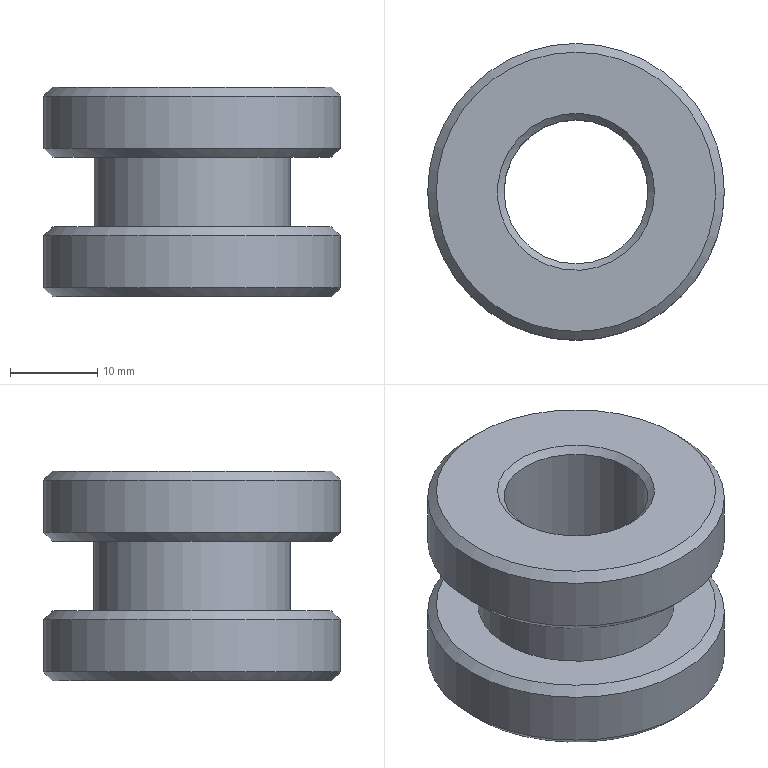Part | STEP file | YBQDJ-PD-16 | 1 solid | 14 faces | box 34 x 34 x 24 mm | volume 12336 mm3 | cone 6 | plane 4 | cylinder 4 | commonest cylinder face diameters 34 x2 16.5 x1 22.5 x1
STEP:
#1=CARTESIAN_POINT('',(0.,0.,0.));
#2=DIRECTION('',(0.,0.,1.));
#3=DIRECTION('',(1.,0.,0.));
#4=AXIS2_PLACEMENT_3D('',#1,#2,#3);
#5=CARTESIAN_POINT('',(-174.5,305.,279.5));
#6=VERTEX_POINT('',#5);
#7=CARTESIAN_POINT('',(-183.5,305.,279.5));
#8=DIRECTION('',(0.,0.,-1.));
#9=DIRECTION('',(1.,0.,0.));
#10=AXIS2_PLACEMENT_3D('',#7,#8,#9);
#11=CIRCLE('',#10,9.);
#12=CARTESIAN_POINT('',(-183.5,305.,279.5));
#13=DIRECTION('',(0.,0.,1.));
#14=DIRECTION('',(1.,0.,0.));
#15=AXIS2_PLACEMENT_3D('',#12,#13,#14);
#16=PLANE('',#15);
#17=CARTESIAN_POINT('',(9.,0.));
#18=CARTESIAN_POINT('',(9.,-15.588));
#19=CARTESIAN_POINT('',(-4.5,-7.794));
#20=CARTESIAN_POINT('',(-18.,0.));
#21=CARTESIAN_POINT('',(-4.5,7.794));
#22=CARTESIAN_POINT('',(9.,15.588));
#23=CARTESIAN_POINT('',(9.,0.));
#24=(BOUNDED_CURVE()B_SPLINE_CURVE(2,(#17,#18,#19,#20,#21,#22,#23),.UNSPECIFIED.,.T.,.F.)B_SPLINE_CURVE_WITH_KNOTS((1,2,2,2,2,1),(-2.094,0.,2.094,4.189,6.283,8.378),.UNSPECIFIED.)CURVE()GEOMETRIC_REPRESENTATION_ITEM()RATIONAL_B_SPLINE_CURVE((1.,0.5,1.,0.5,1.,0.5,1.))REPRESENTATION_ITEM(''));
#25=(GEOMETRIC_REPRESENTATION_CONTEXT(2)PARAMETRIC_REPRESENTATION_CONTEXT()REPRESENTATION_CONTEXT('',''));
#26=DEFINITIONAL_REPRESENTATION('',(#24),#25);
#27=PCURVE('',#16,#26);
#28=CARTESIAN_POINT('',(-183.5,305.,279.5));
#29=DIRECTION('',(0.,0.,1.));
#30=DIRECTION('',(1.,0.,0.));
#31=AXIS2_PLACEMENT_3D('',#28,#29,#30);
#32=CONICAL_SURFACE('',#31,9.,0.7854);
#33=CARTESIAN_POINT('',(6.283,0.));
#34=DIRECTION('',(-1.,0.));
#35=VECTOR('',#34,1.);
#36=LINE('',#33,#35);
#37=(GEOMETRIC_REPRESENTATION_CONTEXT(2)PARAMETRIC_REPRESENTATION_CONTEXT()REPRESENTATION_CONTEXT('',''));
#38=DEFINITIONAL_REPRESENTATION('',(#36),#37);
#39=PCURVE('',#32,#38);
#40=SURFACE_CURVE('',#11,(#27,#39),.PCURVE_S1.);
#41=EDGE_CURVE('',#6,#6,#40,.T.);
#42=ORIENTED_EDGE('',*,*,#41,.T.);
#43=EDGE_LOOP('',(#42));
#44=FACE_BOUND('',#43,.T.);
#45=CARTESIAN_POINT('',(-167.5,305.,279.5));
#46=VERTEX_POINT('',#45);
#47=CARTESIAN_POINT('',(-199.5,305.,279.5));
#48=VERTEX_POINT('',#47);
#49=CARTESIAN_POINT('',(-183.5,305.,279.5));
#50=DIRECTION('',(0.,0.,1.));
#51=DIRECTION('',(1.,0.,0.));
#52=AXIS2_PLACEMENT_3D('',#49,#50,#51);
#53=CIRCLE('',#52,16.);
#54=CARTESIAN_POINT('',(0.,0.));
#55=DIRECTION('',(1.,0.));
#56=AXIS2_PLACEMENT_2D('',#54,#55);
#57=CIRCLE('',#56,16.);
#58=(GEOMETRIC_REPRESENTATION_CONTEXT(2)PARAMETRIC_REPRESENTATION_CONTEXT()REPRESENTATION_CONTEXT('',''));
#59=DEFINITIONAL_REPRESENTATION('',(#57),#58);
#60=PCURVE('',#16,#59);
#61=CARTESIAN_POINT('',(-183.5,305.,279.5));
#62=DIRECTION('',(0.,0.,-1.));
#63=DIRECTION('',(-1.,0.,0.));
#64=AXIS2_PLACEMENT_3D('',#61,#62,#63);
#65=CONICAL_SURFACE('',#64,16.,0.7854);
#66=CARTESIAN_POINT('',(3.142,0.));
#67=DIRECTION('',(-1.,0.));
#68=VECTOR('',#67,1.);
#69=LINE('',#66,#68);
#70=(GEOMETRIC_REPRESENTATION_CONTEXT(2)PARAMETRIC_REPRESENTATION_CONTEXT()REPRESENTATION_CONTEXT('',''));
#71=DEFINITIONAL_REPRESENTATION('',(#69),#70);
#72=PCURVE('',#65,#71);
#73=SURFACE_CURVE('',#53,(#60,#72),.PCURVE_S1.);
#74=EDGE_CURVE('',#46,#48,#73,.T.);
#75=ORIENTED_EDGE('',*,*,#74,.T.);
#76=CARTESIAN_POINT('',(-183.5,305.,279.5));
#77=DIRECTION('',(0.,0.,1.));
#78=DIRECTION('',(1.,0.,0.));
#79=AXIS2_PLACEMENT_3D('',#76,#77,#78);
#80=CIRCLE('',#79,16.);
#81=CARTESIAN_POINT('',(0.,0.));
#82=DIRECTION('',(1.,0.));
#83=AXIS2_PLACEMENT_2D('',#81,#82);
#84=CIRCLE('',#83,16.);
#85=(GEOMETRIC_REPRESENTATION_CONTEXT(2)PARAMETRIC_REPRESENTATION_CONTEXT()REPRESENTATION_CONTEXT('',''));
#86=DEFINITIONAL_REPRESENTATION('',(#84),#85);
#87=PCURVE('',#16,#86);
#88=CARTESIAN_POINT('',(9.425,0.));
#89=DIRECTION('',(-1.,0.));
#90=VECTOR('',#89,1.);
#91=LINE('',#88,#90);
#92=(GEOMETRIC_REPRESENTATION_CONTEXT(2)PARAMETRIC_REPRESENTATION_CONTEXT()REPRESENTATION_CONTEXT('',''));
#93=DEFINITIONAL_REPRESENTATION('',(#91),#92);
#94=PCURVE('',#65,#93);
#95=SURFACE_CURVE('',#80,(#87,#94),.PCURVE_S1.);
#96=EDGE_CURVE('',#48,#46,#95,.T.);
#97=ORIENTED_EDGE('',*,*,#96,.T.);
#98=EDGE_LOOP('',(#75,#97));
#99=FACE_BOUND('',#98,.T.);
#100=ADVANCED_FACE('',(#44,#99),#16,.T.);
#101=CARTESIAN_POINT('',(-174.5,305.,255.5));
#102=VERTEX_POINT('',#101);
#103=CARTESIAN_POINT('',(-183.5,305.,255.5));
#104=DIRECTION('',(0.,0.,1.));
#105=DIRECTION('',(1.,0.,0.));
#106=AXIS2_PLACEMENT_3D('',#103,#104,#105);
#107=CIRCLE('',#106,9.);
#108=CARTESIAN_POINT('',(-183.5,305.,255.5));
#109=DIRECTION('',(0.,0.,1.));
#110=DIRECTION('',(1.,0.,0.));
#111=AXIS2_PLACEMENT_3D('',#108,#109,#110);
#112=PLANE('',#111);
#113=CARTESIAN_POINT('',(0.,0.));
#114=DIRECTION('',(1.,0.));
#115=AXIS2_PLACEMENT_2D('',#113,#114);
#116=CIRCLE('',#115,9.);
#117=(GEOMETRIC_REPRESENTATION_CONTEXT(2)PARAMETRIC_REPRESENTATION_CONTEXT()REPRESENTATION_CONTEXT('',''));
#118=DEFINITIONAL_REPRESENTATION('',(#116),#117);
#119=PCURVE('',#112,#118);
#120=CARTESIAN_POINT('',(-183.5,305.,255.5));
#121=DIRECTION('',(0.,0.,-1.));
#122=DIRECTION('',(-1.,0.,0.));
#123=AXIS2_PLACEMENT_3D('',#120,#121,#122);
#124=CONICAL_SURFACE('',#123,9.,0.7854);
#125=CARTESIAN_POINT('',(9.425,0.));
#126=DIRECTION('',(-1.,0.));
#127=VECTOR('',#126,1.);
#128=LINE('',#125,#127);
#129=(GEOMETRIC_REPRESENTATION_CONTEXT(2)PARAMETRIC_REPRESENTATION_CONTEXT()REPRESENTATION_CONTEXT('',''));
#130=DEFINITIONAL_REPRESENTATION('',(#128),#129);
#131=PCURVE('',#124,#130);
#132=SURFACE_CURVE('',#107,(#119,#131),.PCURVE_S1.);
#133=EDGE_CURVE('',#102,#102,#132,.T.);
#134=ORIENTED_EDGE('',*,*,#133,.T.);
#135=EDGE_LOOP('',(#134));
#136=FACE_BOUND('',#135,.T.);
#137=CARTESIAN_POINT('',(-167.5,305.,255.5));
#138=VERTEX_POINT('',#137);
#139=CARTESIAN_POINT('',(-183.5,305.,255.5));
#140=DIRECTION('',(0.,0.,-1.));
#141=DIRECTION('',(1.,0.,0.));
#142=AXIS2_PLACEMENT_3D('',#139,#140,#141);
#143=CIRCLE('',#142,16.);
#144=CARTESIAN_POINT('',(16.,0.));
#145=CARTESIAN_POINT('',(16.,-27.713));
#146=CARTESIAN_POINT('',(-8.,-13.856));
#147=CARTESIAN_POINT('',(-32.,0.));
#148=CARTESIAN_POINT('',(-8.,13.856));
#149=CARTESIAN_POINT('',(16.,27.713));
#150=CARTESIAN_POINT('',(16.,0.));
#151=(BOUNDED_CURVE()B_SPLINE_CURVE(2,(#144,#145,#146,#147,#148,#149,#150),.UNSPECIFIED.,.T.,.F.)B_SPLINE_CURVE_WITH_KNOTS((1,2,2,2,2,1),(-2.094,0.,2.094,4.189,6.283,8.378),.UNSPECIFIED.)CURVE()GEOMETRIC_REPRESENTATION_ITEM()RATIONAL_B_SPLINE_CURVE((1.,0.5,1.,0.5,1.,0.5,1.))REPRESENTATION_ITEM(''));
#152=(GEOMETRIC_REPRESENTATION_CONTEXT(2)PARAMETRIC_REPRESENTATION_CONTEXT()REPRESENTATION_CONTEXT('',''));
#153=DEFINITIONAL_REPRESENTATION('',(#151),#152);
#154=PCURVE('',#112,#153);
#155=CARTESIAN_POINT('',(-183.5,305.,256.5));
#156=DIRECTION('',(0.,0.,1.));
#157=DIRECTION('',(1.,0.,0.));
#158=AXIS2_PLACEMENT_3D('',#155,#156,#157);
#159=CONICAL_SURFACE('',#158,17.,0.7854);
#160=CARTESIAN_POINT('',(6.283,-1.));
#161=DIRECTION('',(-1.,0.));
#162=VECTOR('',#161,1.);
#163=LINE('',#160,#162);
#164=(GEOMETRIC_REPRESENTATION_CONTEXT(2)PARAMETRIC_REPRESENTATION_CONTEXT()REPRESENTATION_CONTEXT('',''));
#165=DEFINITIONAL_REPRESENTATION('',(#163),#164);
#166=PCURVE('',#159,#165);
#167=SURFACE_CURVE('',#143,(#154,#166),.PCURVE_S1.);
#168=EDGE_CURVE('',#138,#138,#167,.T.);
#169=ORIENTED_EDGE('',*,*,#168,.T.);
#170=EDGE_LOOP('',(#169));
#171=FACE_BOUND('',#170,.T.);
#172=ADVANCED_FACE('',(#136,#171),#112,.F.);
#173=CARTESIAN_POINT('',(-175.25,305.,256.25));
#174=VERTEX_POINT('',#173);
#175=CARTESIAN_POINT('',(-183.5,305.,256.25));
#176=DIRECTION('',(0.,0.,-1.));
#177=DIRECTION('',(1.,0.,0.));
#178=AXIS2_PLACEMENT_3D('',#175,#176,#177);
#179=CIRCLE('',#178,8.25);
#180=CARTESIAN_POINT('',(-183.5,305.,279.5));
#181=DIRECTION('',(0.,0.,-1.));
#182=DIRECTION('',(-1.,0.,0.));
#183=AXIS2_PLACEMENT_3D('',#180,#181,#182);
#184=CYLINDRICAL_SURFACE('',#183,8.25);
#185=CARTESIAN_POINT('',(3.142,23.25));
#186=DIRECTION('',(1.,0.));
#187=VECTOR('',#186,1.);
#188=LINE('',#185,#187);
#189=(GEOMETRIC_REPRESENTATION_CONTEXT(2)PARAMETRIC_REPRESENTATION_CONTEXT()REPRESENTATION_CONTEXT('',''));
#190=DEFINITIONAL_REPRESENTATION('',(#188),#189);
#191=PCURVE('',#184,#190);
#192=CARTESIAN_POINT('',(3.142,-0.75));
#193=DIRECTION('',(1.,0.));
#194=VECTOR('',#193,1.);
#195=LINE('',#192,#194);
#196=(GEOMETRIC_REPRESENTATION_CONTEXT(2)PARAMETRIC_REPRESENTATION_CONTEXT()REPRESENTATION_CONTEXT('',''));
#197=DEFINITIONAL_REPRESENTATION('',(#195),#196);
#198=PCURVE('',#124,#197);
#199=SURFACE_CURVE('',#179,(#191,#198),.PCURVE_S1.);
#200=EDGE_CURVE('',#174,#174,#199,.T.);
#201=ORIENTED_EDGE('',*,*,#200,.F.);
#202=CARTESIAN_POINT('',(-175.25,305.,278.75));
#203=VERTEX_POINT('',#202);
#204=CARTESIAN_POINT('',(-175.25,305.,278.75));
#205=CARTESIAN_POINT('',(-175.25,305.,256.25));
#206=B_SPLINE_CURVE_WITH_KNOTS('',1,(#204,#205),.UNSPECIFIED.,.F.,.F.,(2,2),(0.75,23.25),.PIECEWISE_BEZIER_KNOTS.);
#207=CARTESIAN_POINT('',(3.142,0.));
#208=DIRECTION('',(0.,1.));
#209=VECTOR('',#208,1.);
#210=LINE('',#207,#209);
#211=(GEOMETRIC_REPRESENTATION_CONTEXT(2)PARAMETRIC_REPRESENTATION_CONTEXT()REPRESENTATION_CONTEXT('',''));
#212=DEFINITIONAL_REPRESENTATION('',(#210),#211);
#213=PCURVE('',#184,#212);
#214=CARTESIAN_POINT('',(9.425,0.));
#215=DIRECTION('',(0.,1.));
#216=VECTOR('',#215,1.);
#217=LINE('',#214,#216);
#218=(GEOMETRIC_REPRESENTATION_CONTEXT(2)PARAMETRIC_REPRESENTATION_CONTEXT()REPRESENTATION_CONTEXT('',''));
#219=DEFINITIONAL_REPRESENTATION('',(#217),#218);
#220=PCURVE('',#184,#219);
#221=SEAM_CURVE('',#206,(#213,#220),.PCURVE_S1.);
#222=EDGE_CURVE('',#203,#174,#221,.T.);
#223=ORIENTED_EDGE('',*,*,#222,.F.);
#224=CARTESIAN_POINT('',(-183.5,305.,278.75));
#225=DIRECTION('',(0.,0.,1.));
#226=DIRECTION('',(1.,0.,0.));
#227=AXIS2_PLACEMENT_3D('',#224,#225,#226);
#228=CIRCLE('',#227,8.25);
#229=CARTESIAN_POINT('',(9.425,0.75));
#230=DIRECTION('',(-1.,0.));
#231=VECTOR('',#230,1.);
#232=LINE('',#229,#231);
#233=(GEOMETRIC_REPRESENTATION_CONTEXT(2)PARAMETRIC_REPRESENTATION_CONTEXT()REPRESENTATION_CONTEXT('',''));
#234=DEFINITIONAL_REPRESENTATION('',(#232),#233);
#235=PCURVE('',#184,#234);
#236=CARTESIAN_POINT('',(0.,-0.75));
#237=DIRECTION('',(1.,0.));
#238=VECTOR('',#237,1.);
#239=LINE('',#236,#238);
#240=(GEOMETRIC_REPRESENTATION_CONTEXT(2)PARAMETRIC_REPRESENTATION_CONTEXT()REPRESENTATION_CONTEXT('',''));
#241=DEFINITIONAL_REPRESENTATION('',(#239),#240);
#242=PCURVE('',#32,#241);
#243=SURFACE_CURVE('',#228,(#235,#242),.PCURVE_S1.);
#244=EDGE_CURVE('',#203,#203,#243,.T.);
#245=ORIENTED_EDGE('',*,*,#244,.F.);
#246=ORIENTED_EDGE('',*,*,#222,.T.);
#247=EDGE_LOOP('',(#201,#223,#245,#246));
#248=FACE_BOUND('',#247,.F.);
#249=ADVANCED_FACE('',(#248),#184,.F.);
#250=CARTESIAN_POINT('',(-166.5,305.,272.5));
#251=VERTEX_POINT('',#250);
#252=CARTESIAN_POINT('',(-200.5,305.,272.5));
#253=VERTEX_POINT('',#252);
#254=CARTESIAN_POINT('',(-183.5,305.,272.5));
#255=DIRECTION('',(0.,0.,1.));
#256=DIRECTION('',(1.,0.,0.));
#257=AXIS2_PLACEMENT_3D('',#254,#255,#256);
#258=CIRCLE('',#257,17.);
#259=CARTESIAN_POINT('',(-183.5,305.,279.5));
#260=DIRECTION('',(0.,0.,-1.));
#261=DIRECTION('',(-1.,0.,0.));
#262=AXIS2_PLACEMENT_3D('',#259,#260,#261);
#263=CYLINDRICAL_SURFACE('',#262,17.);
#264=CARTESIAN_POINT('',(3.142,7.));
#265=DIRECTION('',(-1.,0.));
#266=VECTOR('',#265,1.);
#267=LINE('',#264,#266);
#268=(GEOMETRIC_REPRESENTATION_CONTEXT(2)PARAMETRIC_REPRESENTATION_CONTEXT()REPRESENTATION_CONTEXT('',''));
#269=DEFINITIONAL_REPRESENTATION('',(#267),#268);
#270=PCURVE('',#263,#269);
#271=CARTESIAN_POINT('',(-183.5,305.,272.5));
#272=DIRECTION('',(0.,0.,1.));
#273=DIRECTION('',(1.,0.,0.));
#274=AXIS2_PLACEMENT_3D('',#271,#272,#273);
#275=CONICAL_SURFACE('',#274,17.,0.7854);
#276=CARTESIAN_POINT('',(0.,0.));
#277=DIRECTION('',(1.,0.));
#278=VECTOR('',#277,1.);
#279=LINE('',#276,#278);
#280=(GEOMETRIC_REPRESENTATION_CONTEXT(2)PARAMETRIC_REPRESENTATION_CONTEXT()REPRESENTATION_CONTEXT('',''));
#281=DEFINITIONAL_REPRESENTATION('',(#279),#280);
#282=PCURVE('',#275,#281);
#283=SURFACE_CURVE('',#258,(#270,#282),.PCURVE_S1.);
#284=EDGE_CURVE('',#251,#253,#283,.T.);
#285=ORIENTED_EDGE('',*,*,#284,.T.);
#286=CARTESIAN_POINT('',(-200.5,305.,278.5));
#287=VERTEX_POINT('',#286);
#288=CARTESIAN_POINT('',(-200.5,305.,278.5));
#289=CARTESIAN_POINT('',(-200.5,305.,272.5));
#290=B_SPLINE_CURVE_WITH_KNOTS('',1,(#288,#289),.UNSPECIFIED.,.F.,.F.,(2,2),(1.,7.),.PIECEWISE_BEZIER_KNOTS.);
#291=CARTESIAN_POINT('',(0.,0.));
#292=DIRECTION('',(0.,1.));
#293=VECTOR('',#292,1.);
#294=LINE('',#291,#293);
#295=(GEOMETRIC_REPRESENTATION_CONTEXT(2)PARAMETRIC_REPRESENTATION_CONTEXT()REPRESENTATION_CONTEXT('',''));
#296=DEFINITIONAL_REPRESENTATION('',(#294),#295);
#297=PCURVE('',#263,#296);
#298=CARTESIAN_POINT('',(6.283,0.));
#299=DIRECTION('',(0.,1.));
#300=VECTOR('',#299,1.);
#301=LINE('',#298,#300);
#302=(GEOMETRIC_REPRESENTATION_CONTEXT(2)PARAMETRIC_REPRESENTATION_CONTEXT()REPRESENTATION_CONTEXT('',''));
#303=DEFINITIONAL_REPRESENTATION('',(#301),#302);
#304=PCURVE('',#263,#303);
#305=SEAM_CURVE('',#290,(#297,#304),.PCURVE_S1.);
#306=EDGE_CURVE('',#287,#253,#305,.T.);
#307=ORIENTED_EDGE('',*,*,#306,.F.);
#308=CARTESIAN_POINT('',(-183.5,305.,278.5));
#309=DIRECTION('',(0.,0.,-1.));
#310=DIRECTION('',(-1.,0.,0.));
#311=AXIS2_PLACEMENT_3D('',#308,#309,#310);
#312=CIRCLE('',#311,17.);
#313=CARTESIAN_POINT('',(0.,1.));
#314=DIRECTION('',(1.,0.));
#315=VECTOR('',#314,1.);
#316=LINE('',#313,#315);
#317=(GEOMETRIC_REPRESENTATION_CONTEXT(2)PARAMETRIC_REPRESENTATION_CONTEXT()REPRESENTATION_CONTEXT('',''));
#318=DEFINITIONAL_REPRESENTATION('',(#316),#317);
#319=PCURVE('',#263,#318);
#320=CARTESIAN_POINT('',(0.,1.));
#321=DIRECTION('',(1.,0.));
#322=VECTOR('',#321,1.);
#323=LINE('',#320,#322);
#324=(GEOMETRIC_REPRESENTATION_CONTEXT(2)PARAMETRIC_REPRESENTATION_CONTEXT()REPRESENTATION_CONTEXT('',''));
#325=DEFINITIONAL_REPRESENTATION('',(#323),#324);
#326=PCURVE('',#65,#325);
#327=SURFACE_CURVE('',#312,(#319,#326),.PCURVE_S1.);
#328=EDGE_CURVE('',#287,#287,#327,.T.);
#329=ORIENTED_EDGE('',*,*,#328,.T.);
#330=ORIENTED_EDGE('',*,*,#306,.T.);
#331=CARTESIAN_POINT('',(-183.5,305.,272.5));
#332=DIRECTION('',(0.,0.,1.));
#333=DIRECTION('',(1.,0.,0.));
#334=AXIS2_PLACEMENT_3D('',#331,#332,#333);
#335=CIRCLE('',#334,17.);
#336=CARTESIAN_POINT('',(9.425,7.));
#337=DIRECTION('',(-1.,0.));
#338=VECTOR('',#337,1.);
#339=LINE('',#336,#338);
#340=(GEOMETRIC_REPRESENTATION_CONTEXT(2)PARAMETRIC_REPRESENTATION_CONTEXT()REPRESENTATION_CONTEXT('',''));
#341=DEFINITIONAL_REPRESENTATION('',(#339),#340);
#342=PCURVE('',#263,#341);
#343=CARTESIAN_POINT('',(0.,0.));
#344=DIRECTION('',(1.,0.));
#345=VECTOR('',#344,1.);
#346=LINE('',#343,#345);
#347=(GEOMETRIC_REPRESENTATION_CONTEXT(2)PARAMETRIC_REPRESENTATION_CONTEXT()REPRESENTATION_CONTEXT('',''));
#348=DEFINITIONAL_REPRESENTATION('',(#346),#347);
#349=PCURVE('',#275,#348);
#350=SURFACE_CURVE('',#335,(#342,#349),.PCURVE_S1.);
#351=EDGE_CURVE('',#253,#251,#350,.T.);
#352=ORIENTED_EDGE('',*,*,#351,.T.);
#353=EDGE_LOOP('',(#285,#307,#329,#330,#352));
#354=FACE_BOUND('',#353,.T.);
#355=ADVANCED_FACE('',(#354),#263,.T.);
#356=CARTESIAN_POINT('',(-167.5,305.,271.5));
#357=VERTEX_POINT('',#356);
#358=CARTESIAN_POINT('',(-183.5,305.,271.5));
#359=DIRECTION('',(0.,0.,-1.));
#360=DIRECTION('',(1.,0.,0.));
#361=AXIS2_PLACEMENT_3D('',#358,#359,#360);
#362=CIRCLE('',#361,16.);
#363=CARTESIAN_POINT('',(-183.5,305.,271.5));
#364=DIRECTION('',(0.,0.,1.));
#365=DIRECTION('',(1.,0.,0.));
#366=AXIS2_PLACEMENT_3D('',#363,#364,#365);
#367=PLANE('',#366);
#368=CARTESIAN_POINT('',(16.,0.));
#369=CARTESIAN_POINT('',(16.,-27.713));
#370=CARTESIAN_POINT('',(-8.,-13.856));
#371=CARTESIAN_POINT('',(-32.,0.));
#372=CARTESIAN_POINT('',(-8.,13.856));
#373=CARTESIAN_POINT('',(16.,27.713));
#374=CARTESIAN_POINT('',(16.,0.));
#375=(BOUNDED_CURVE()B_SPLINE_CURVE(2,(#368,#369,#370,#371,#372,#373,#374),.UNSPECIFIED.,.T.,.F.)B_SPLINE_CURVE_WITH_KNOTS((1,2,2,2,2,1),(-2.094,0.,2.094,4.189,6.283,8.378),.UNSPECIFIED.)CURVE()GEOMETRIC_REPRESENTATION_ITEM()RATIONAL_B_SPLINE_CURVE((1.,0.5,1.,0.5,1.,0.5,1.))REPRESENTATION_ITEM(''));
#376=(GEOMETRIC_REPRESENTATION_CONTEXT(2)PARAMETRIC_REPRESENTATION_CONTEXT()REPRESENTATION_CONTEXT('',''));
#377=DEFINITIONAL_REPRESENTATION('',(#375),#376);
#378=PCURVE('',#367,#377);
#379=CARTESIAN_POINT('',(6.283,-1.));
#380=DIRECTION('',(-1.,0.));
#381=VECTOR('',#380,1.);
#382=LINE('',#379,#381);
#383=(GEOMETRIC_REPRESENTATION_CONTEXT(2)PARAMETRIC_REPRESENTATION_CONTEXT()REPRESENTATION_CONTEXT('',''));
#384=DEFINITIONAL_REPRESENTATION('',(#382),#383);
#385=PCURVE('',#275,#384);
#386=SURFACE_CURVE('',#362,(#378,#385),.PCURVE_S1.);
#387=EDGE_CURVE('',#357,#357,#386,.T.);
#388=ORIENTED_EDGE('',*,*,#387,.T.);
#389=EDGE_LOOP('',(#388));
#390=FACE_BOUND('',#389,.T.);
#391=CARTESIAN_POINT('',(-172.25,305.,271.5));
#392=VERTEX_POINT('',#391);
#393=CARTESIAN_POINT('',(-183.5,305.,271.5));
#394=DIRECTION('',(0.,0.,1.));
#395=DIRECTION('',(1.,0.,0.));
#396=AXIS2_PLACEMENT_3D('',#393,#394,#395);
#397=CIRCLE('',#396,11.25);
#398=CARTESIAN_POINT('',(0.,0.));
#399=DIRECTION('',(1.,0.));
#400=AXIS2_PLACEMENT_2D('',#398,#399);
#401=CIRCLE('',#400,11.25);
#402=(GEOMETRIC_REPRESENTATION_CONTEXT(2)PARAMETRIC_REPRESENTATION_CONTEXT()REPRESENTATION_CONTEXT('',''));
#403=DEFINITIONAL_REPRESENTATION('',(#401),#402);
#404=PCURVE('',#367,#403);
#405=CARTESIAN_POINT('',(-183.5,305.,271.5));
#406=DIRECTION('',(0.,0.,-1.));
#407=DIRECTION('',(-1.,0.,0.));
#408=AXIS2_PLACEMENT_3D('',#405,#406,#407);
#409=CYLINDRICAL_SURFACE('',#408,11.25);
#410=CARTESIAN_POINT('',(9.425,0.));
#411=DIRECTION('',(-1.,0.));
#412=VECTOR('',#411,1.);
#413=LINE('',#410,#412);
#414=(GEOMETRIC_REPRESENTATION_CONTEXT(2)PARAMETRIC_REPRESENTATION_CONTEXT()REPRESENTATION_CONTEXT('',''));
#415=DEFINITIONAL_REPRESENTATION('',(#413),#414);
#416=PCURVE('',#409,#415);
#417=SURFACE_CURVE('',#397,(#404,#416),.PCURVE_S1.);
#418=EDGE_CURVE('',#392,#392,#417,.T.);
#419=ORIENTED_EDGE('',*,*,#418,.T.);
#420=EDGE_LOOP('',(#419));
#421=FACE_BOUND('',#420,.T.);
#422=ADVANCED_FACE('',(#390,#421),#367,.F.);
#423=CARTESIAN_POINT('',(-166.5,305.,256.5));
#424=VERTEX_POINT('',#423);
#425=CARTESIAN_POINT('',(-200.5,305.,256.5));
#426=VERTEX_POINT('',#425);
#427=CARTESIAN_POINT('',(-183.5,305.,256.5));
#428=DIRECTION('',(0.,0.,1.));
#429=DIRECTION('',(1.,0.,0.));
#430=AXIS2_PLACEMENT_3D('',#427,#428,#429);
#431=CIRCLE('',#430,17.);
#432=CARTESIAN_POINT('',(-183.5,305.,263.5));
#433=DIRECTION('',(0.,0.,-1.));
#434=DIRECTION('',(-1.,0.,0.));
#435=AXIS2_PLACEMENT_3D('',#432,#433,#434);
#436=CYLINDRICAL_SURFACE('',#435,17.);
#437=CARTESIAN_POINT('',(3.142,7.));
#438=DIRECTION('',(-1.,0.));
#439=VECTOR('',#438,1.);
#440=LINE('',#437,#439);
#441=(GEOMETRIC_REPRESENTATION_CONTEXT(2)PARAMETRIC_REPRESENTATION_CONTEXT()REPRESENTATION_CONTEXT('',''));
#442=DEFINITIONAL_REPRESENTATION('',(#440),#441);
#443=PCURVE('',#436,#442);
#444=CARTESIAN_POINT('',(0.,0.));
#445=DIRECTION('',(1.,0.));
#446=VECTOR('',#445,1.);
#447=LINE('',#444,#446);
#448=(GEOMETRIC_REPRESENTATION_CONTEXT(2)PARAMETRIC_REPRESENTATION_CONTEXT()REPRESENTATION_CONTEXT('',''));
#449=DEFINITIONAL_REPRESENTATION('',(#447),#448);
#450=PCURVE('',#159,#449);
#451=SURFACE_CURVE('',#431,(#443,#450),.PCURVE_S1.);
#452=EDGE_CURVE('',#424,#426,#451,.T.);
#453=ORIENTED_EDGE('',*,*,#452,.T.);
#454=CARTESIAN_POINT('',(-200.5,305.,262.5));
#455=VERTEX_POINT('',#454);
#456=CARTESIAN_POINT('',(-200.5,305.,262.5));
#457=CARTESIAN_POINT('',(-200.5,305.,256.5));
#458=B_SPLINE_CURVE_WITH_KNOTS('',1,(#456,#457),.UNSPECIFIED.,.F.,.F.,(2,2),(1.,7.),.PIECEWISE_BEZIER_KNOTS.);
#459=CARTESIAN_POINT('',(0.,0.));
#460=DIRECTION('',(0.,1.));
#461=VECTOR('',#460,1.);
#462=LINE('',#459,#461);
#463=(GEOMETRIC_REPRESENTATION_CONTEXT(2)PARAMETRIC_REPRESENTATION_CONTEXT()REPRESENTATION_CONTEXT('',''));
#464=DEFINITIONAL_REPRESENTATION('',(#462),#463);
#465=PCURVE('',#436,#464);
#466=CARTESIAN_POINT('',(6.283,0.));
#467=DIRECTION('',(0.,1.));
#468=VECTOR('',#467,1.);
#469=LINE('',#466,#468);
#470=(GEOMETRIC_REPRESENTATION_CONTEXT(2)PARAMETRIC_REPRESENTATION_CONTEXT()REPRESENTATION_CONTEXT('',''));
#471=DEFINITIONAL_REPRESENTATION('',(#469),#470);
#472=PCURVE('',#436,#471);
#473=SEAM_CURVE('',#458,(#465,#472),.PCURVE_S1.);
#474=EDGE_CURVE('',#455,#426,#473,.T.);
#475=ORIENTED_EDGE('',*,*,#474,.F.);
#476=CARTESIAN_POINT('',(-183.5,305.,262.5));
#477=DIRECTION('',(0.,0.,-1.));
#478=DIRECTION('',(-1.,0.,0.));
#479=AXIS2_PLACEMENT_3D('',#476,#477,#478);
#480=CIRCLE('',#479,17.);
#481=CARTESIAN_POINT('',(0.,1.));
#482=DIRECTION('',(1.,0.));
#483=VECTOR('',#482,1.);
#484=LINE('',#481,#483);
#485=(GEOMETRIC_REPRESENTATION_CONTEXT(2)PARAMETRIC_REPRESENTATION_CONTEXT()REPRESENTATION_CONTEXT('',''));
#486=DEFINITIONAL_REPRESENTATION('',(#484),#485);
#487=PCURVE('',#436,#486);
#488=CARTESIAN_POINT('',(-183.5,305.,263.5));
#489=DIRECTION('',(0.,0.,-1.));
#490=DIRECTION('',(-1.,0.,0.));
#491=AXIS2_PLACEMENT_3D('',#488,#489,#490);
#492=CONICAL_SURFACE('',#491,16.,0.7854);
#493=CARTESIAN_POINT('',(0.,1.));
#494=DIRECTION('',(1.,0.));
#495=VECTOR('',#494,1.);
#496=LINE('',#493,#495);
#497=(GEOMETRIC_REPRESENTATION_CONTEXT(2)PARAMETRIC_REPRESENTATION_CONTEXT()REPRESENTATION_CONTEXT('',''));
#498=DEFINITIONAL_REPRESENTATION('',(#496),#497);
#499=PCURVE('',#492,#498);
#500=SURFACE_CURVE('',#480,(#487,#499),.PCURVE_S1.);
#501=EDGE_CURVE('',#455,#455,#500,.T.);
#502=ORIENTED_EDGE('',*,*,#501,.T.);
#503=ORIENTED_EDGE('',*,*,#474,.T.);
#504=CARTESIAN_POINT('',(-183.5,305.,256.5));
#505=DIRECTION('',(0.,0.,1.));
#506=DIRECTION('',(1.,0.,0.));
#507=AXIS2_PLACEMENT_3D('',#504,#505,#506);
#508=CIRCLE('',#507,17.);
#509=CARTESIAN_POINT('',(9.425,7.));
#510=DIRECTION('',(-1.,0.));
#511=VECTOR('',#510,1.);
#512=LINE('',#509,#511);
#513=(GEOMETRIC_REPRESENTATION_CONTEXT(2)PARAMETRIC_REPRESENTATION_CONTEXT()REPRESENTATION_CONTEXT('',''));
#514=DEFINITIONAL_REPRESENTATION('',(#512),#513);
#515=PCURVE('',#436,#514);
#516=CARTESIAN_POINT('',(0.,0.));
#517=DIRECTION('',(1.,0.));
#518=VECTOR('',#517,1.);
#519=LINE('',#516,#518);
#520=(GEOMETRIC_REPRESENTATION_CONTEXT(2)PARAMETRIC_REPRESENTATION_CONTEXT()REPRESENTATION_CONTEXT('',''));
#521=DEFINITIONAL_REPRESENTATION('',(#519),#520);
#522=PCURVE('',#159,#521);
#523=SURFACE_CURVE('',#508,(#515,#522),.PCURVE_S1.);
#524=EDGE_CURVE('',#426,#424,#523,.T.);
#525=ORIENTED_EDGE('',*,*,#524,.T.);
#526=EDGE_LOOP('',(#453,#475,#502,#503,#525));
#527=FACE_BOUND('',#526,.T.);
#528=ADVANCED_FACE('',(#527),#436,.T.);
#529=CARTESIAN_POINT('',(-167.5,305.,263.5));
#530=VERTEX_POINT('',#529);
#531=CARTESIAN_POINT('',(-199.5,305.,263.5));
#532=VERTEX_POINT('',#531);
#533=CARTESIAN_POINT('',(-183.5,305.,263.5));
#534=DIRECTION('',(0.,0.,1.));
#535=DIRECTION('',(1.,0.,0.));
#536=AXIS2_PLACEMENT_3D('',#533,#534,#535);
#537=CIRCLE('',#536,16.);
#538=CARTESIAN_POINT('',(-183.5,305.,263.5));
#539=DIRECTION('',(0.,0.,1.));
#540=DIRECTION('',(1.,0.,0.));
#541=AXIS2_PLACEMENT_3D('',#538,#539,#540);
#542=PLANE('',#541);
#543=CARTESIAN_POINT('',(0.,0.));
#544=DIRECTION('',(1.,0.));
#545=AXIS2_PLACEMENT_2D('',#543,#544);
#546=CIRCLE('',#545,16.);
#547=(GEOMETRIC_REPRESENTATION_CONTEXT(2)PARAMETRIC_REPRESENTATION_CONTEXT()REPRESENTATION_CONTEXT('',''));
#548=DEFINITIONAL_REPRESENTATION('',(#546),#547);
#549=PCURVE('',#542,#548);
#550=CARTESIAN_POINT('',(3.142,0.));
#551=DIRECTION('',(-1.,0.));
#552=VECTOR('',#551,1.);
#553=LINE('',#550,#552);
#554=(GEOMETRIC_REPRESENTATION_CONTEXT(2)PARAMETRIC_REPRESENTATION_CONTEXT()REPRESENTATION_CONTEXT('',''));
#555=DEFINITIONAL_REPRESENTATION('',(#553),#554);
#556=PCURVE('',#492,#555);
#557=SURFACE_CURVE('',#537,(#549,#556),.PCURVE_S1.);
#558=EDGE_CURVE('',#530,#532,#557,.T.);
#559=ORIENTED_EDGE('',*,*,#558,.T.);
#560=CARTESIAN_POINT('',(-183.5,305.,263.5));
#561=DIRECTION('',(0.,0.,1.));
#562=DIRECTION('',(1.,0.,0.));
#563=AXIS2_PLACEMENT_3D('',#560,#561,#562);
#564=CIRCLE('',#563,16.);
#565=CARTESIAN_POINT('',(0.,0.));
#566=DIRECTION('',(1.,0.));
#567=AXIS2_PLACEMENT_2D('',#565,#566);
#568=CIRCLE('',#567,16.);
#569=(GEOMETRIC_REPRESENTATION_CONTEXT(2)PARAMETRIC_REPRESENTATION_CONTEXT()REPRESENTATION_CONTEXT('',''));
#570=DEFINITIONAL_REPRESENTATION('',(#568),#569);
#571=PCURVE('',#542,#570);
#572=CARTESIAN_POINT('',(9.425,0.));
#573=DIRECTION('',(-1.,0.));
#574=VECTOR('',#573,1.);
#575=LINE('',#572,#574);
#576=(GEOMETRIC_REPRESENTATION_CONTEXT(2)PARAMETRIC_REPRESENTATION_CONTEXT()REPRESENTATION_CONTEXT('',''));
#577=DEFINITIONAL_REPRESENTATION('',(#575),#576);
#578=PCURVE('',#492,#577);
#579=SURFACE_CURVE('',#564,(#571,#578),.PCURVE_S1.);
#580=EDGE_CURVE('',#532,#530,#579,.T.);
#581=ORIENTED_EDGE('',*,*,#580,.T.);
#582=EDGE_LOOP('',(#559,#581));
#583=FACE_BOUND('',#582,.T.);
#584=CARTESIAN_POINT('',(-172.25,305.,263.5));
#585=VERTEX_POINT('',#584);
#586=CARTESIAN_POINT('',(-183.5,305.,263.5));
#587=DIRECTION('',(0.,0.,1.));
#588=DIRECTION('',(1.,0.,0.));
#589=AXIS2_PLACEMENT_3D('',#586,#587,#588);
#590=CIRCLE('',#589,11.25);
#591=CARTESIAN_POINT('',(0.,0.));
#592=DIRECTION('',(1.,0.));
#593=AXIS2_PLACEMENT_2D('',#591,#592);
#594=CIRCLE('',#593,11.25);
#595=(GEOMETRIC_REPRESENTATION_CONTEXT(2)PARAMETRIC_REPRESENTATION_CONTEXT()REPRESENTATION_CONTEXT('',''));
#596=DEFINITIONAL_REPRESENTATION('',(#594),#595);
#597=PCURVE('',#542,#596);
#598=CARTESIAN_POINT('',(9.425,8.));
#599=DIRECTION('',(-1.,0.));
#600=VECTOR('',#599,1.);
#601=LINE('',#598,#600);
#602=(GEOMETRIC_REPRESENTATION_CONTEXT(2)PARAMETRIC_REPRESENTATION_CONTEXT()REPRESENTATION_CONTEXT('',''));
#603=DEFINITIONAL_REPRESENTATION('',(#601),#602);
#604=PCURVE('',#409,#603);
#605=SURFACE_CURVE('',#590,(#597,#604),.PCURVE_S1.);
#606=EDGE_CURVE('',#585,#585,#605,.T.);
#607=ORIENTED_EDGE('',*,*,#606,.F.);
#608=EDGE_LOOP('',(#607));
#609=FACE_BOUND('',#608,.T.);
#610=ADVANCED_FACE('',(#583,#609),#542,.T.);
#611=ORIENTED_EDGE('',*,*,#418,.F.);
#612=CARTESIAN_POINT('',(-172.25,305.,271.5));
#613=CARTESIAN_POINT('',(-172.25,305.,263.5));
#614=B_SPLINE_CURVE_WITH_KNOTS('',1,(#612,#613),.UNSPECIFIED.,.F.,.F.,(2,2),(0.,8.),.PIECEWISE_BEZIER_KNOTS.);
#615=CARTESIAN_POINT('',(9.425,0.));
#616=DIRECTION('',(0.,1.));
#617=VECTOR('',#616,1.);
#618=LINE('',#615,#617);
#619=(GEOMETRIC_REPRESENTATION_CONTEXT(2)PARAMETRIC_REPRESENTATION_CONTEXT()REPRESENTATION_CONTEXT('',''));
#620=DEFINITIONAL_REPRESENTATION('',(#618),#619);
#621=PCURVE('',#409,#620);
#622=CARTESIAN_POINT('',(3.142,0.));
#623=DIRECTION('',(0.,1.));
#624=VECTOR('',#623,1.);
#625=LINE('',#622,#624);
#626=(GEOMETRIC_REPRESENTATION_CONTEXT(2)PARAMETRIC_REPRESENTATION_CONTEXT()REPRESENTATION_CONTEXT('',''));
#627=DEFINITIONAL_REPRESENTATION('',(#625),#626);
#628=PCURVE('',#409,#627);
#629=SEAM_CURVE('',#614,(#621,#628),.PCURVE_S1.);
#630=EDGE_CURVE('',#392,#585,#629,.T.);
#631=ORIENTED_EDGE('',*,*,#630,.T.);
#632=ORIENTED_EDGE('',*,*,#606,.T.);
#633=ORIENTED_EDGE('',*,*,#630,.F.);
#634=EDGE_LOOP('',(#611,#631,#632,#633));
#635=FACE_BOUND('',#634,.T.);
#636=ADVANCED_FACE('',(#635),#409,.T.);
#637=ORIENTED_EDGE('',*,*,#168,.F.);
#638=CARTESIAN_POINT('',(-167.5,305.,255.5));
#639=CARTESIAN_POINT('',(-166.5,305.,256.5));
#640=B_SPLINE_CURVE_WITH_KNOTS('',1,(#638,#639),.UNSPECIFIED.,.F.,.F.,(2,2),(-1.414,0.),.PIECEWISE_BEZIER_KNOTS.);
#641=CARTESIAN_POINT('',(6.283,0.));
#642=DIRECTION('',(0.,1.));
#643=VECTOR('',#642,1.);
#644=LINE('',#641,#643);
#645=(GEOMETRIC_REPRESENTATION_CONTEXT(2)PARAMETRIC_REPRESENTATION_CONTEXT()REPRESENTATION_CONTEXT('',''));
#646=DEFINITIONAL_REPRESENTATION('',(#644),#645);
#647=PCURVE('',#159,#646);
#648=CARTESIAN_POINT('',(0.,0.));
#649=DIRECTION('',(0.,1.));
#650=VECTOR('',#649,1.);
#651=LINE('',#648,#650);
#652=(GEOMETRIC_REPRESENTATION_CONTEXT(2)PARAMETRIC_REPRESENTATION_CONTEXT()REPRESENTATION_CONTEXT('',''));
#653=DEFINITIONAL_REPRESENTATION('',(#651),#652);
#654=PCURVE('',#159,#653);
#655=SEAM_CURVE('',#640,(#647,#654),.PCURVE_S1.);
#656=EDGE_CURVE('',#138,#424,#655,.T.);
#657=ORIENTED_EDGE('',*,*,#656,.T.);
#658=ORIENTED_EDGE('',*,*,#524,.F.);
#659=ORIENTED_EDGE('',*,*,#452,.F.);
#660=ORIENTED_EDGE('',*,*,#656,.F.);
#661=EDGE_LOOP('',(#637,#657,#658,#659,#660));
#662=FACE_BOUND('',#661,.T.);
#663=ADVANCED_FACE('',(#662),#159,.T.);
#664=ORIENTED_EDGE('',*,*,#501,.F.);
#665=CARTESIAN_POINT('',(-199.5,305.,263.5));
#666=CARTESIAN_POINT('',(-200.5,305.,262.5));
#667=B_SPLINE_CURVE_WITH_KNOTS('',1,(#665,#666),.UNSPECIFIED.,.F.,.F.,(2,2),(0.,1.414),.PIECEWISE_BEZIER_KNOTS.);
#668=CARTESIAN_POINT('',(0.,0.));
#669=DIRECTION('',(0.,1.));
#670=VECTOR('',#669,1.);
#671=LINE('',#668,#670);
#672=(GEOMETRIC_REPRESENTATION_CONTEXT(2)PARAMETRIC_REPRESENTATION_CONTEXT()REPRESENTATION_CONTEXT('',''));
#673=DEFINITIONAL_REPRESENTATION('',(#671),#672);
#674=PCURVE('',#492,#673);
#675=CARTESIAN_POINT('',(6.283,0.));
#676=DIRECTION('',(0.,1.));
#677=VECTOR('',#676,1.);
#678=LINE('',#675,#677);
#679=(GEOMETRIC_REPRESENTATION_CONTEXT(2)PARAMETRIC_REPRESENTATION_CONTEXT()REPRESENTATION_CONTEXT('',''));
#680=DEFINITIONAL_REPRESENTATION('',(#678),#679);
#681=PCURVE('',#492,#680);
#682=SEAM_CURVE('',#667,(#674,#681),.PCURVE_S1.);
#683=EDGE_CURVE('',#532,#455,#682,.T.);
#684=ORIENTED_EDGE('',*,*,#683,.F.);
#685=ORIENTED_EDGE('',*,*,#558,.F.);
#686=ORIENTED_EDGE('',*,*,#580,.F.);
#687=ORIENTED_EDGE('',*,*,#683,.T.);
#688=EDGE_LOOP('',(#664,#684,#685,#686,#687));
#689=FACE_BOUND('',#688,.T.);
#690=ADVANCED_FACE('',(#689),#492,.T.);
#691=ORIENTED_EDGE('',*,*,#387,.F.);
#692=CARTESIAN_POINT('',(-167.5,305.,271.5));
#693=CARTESIAN_POINT('',(-166.5,305.,272.5));
#694=B_SPLINE_CURVE_WITH_KNOTS('',1,(#692,#693),.UNSPECIFIED.,.F.,.F.,(2,2),(-1.414,0.),.PIECEWISE_BEZIER_KNOTS.);
#695=CARTESIAN_POINT('',(6.283,0.));
#696=DIRECTION('',(0.,1.));
#697=VECTOR('',#696,1.);
#698=LINE('',#695,#697);
#699=(GEOMETRIC_REPRESENTATION_CONTEXT(2)PARAMETRIC_REPRESENTATION_CONTEXT()REPRESENTATION_CONTEXT('',''));
#700=DEFINITIONAL_REPRESENTATION('',(#698),#699);
#701=PCURVE('',#275,#700);
#702=CARTESIAN_POINT('',(0.,0.));
#703=DIRECTION('',(0.,1.));
#704=VECTOR('',#703,1.);
#705=LINE('',#702,#704);
#706=(GEOMETRIC_REPRESENTATION_CONTEXT(2)PARAMETRIC_REPRESENTATION_CONTEXT()REPRESENTATION_CONTEXT('',''));
#707=DEFINITIONAL_REPRESENTATION('',(#705),#706);
#708=PCURVE('',#275,#707);
#709=SEAM_CURVE('',#694,(#701,#708),.PCURVE_S1.);
#710=EDGE_CURVE('',#357,#251,#709,.T.);
#711=ORIENTED_EDGE('',*,*,#710,.T.);
#712=ORIENTED_EDGE('',*,*,#351,.F.);
#713=ORIENTED_EDGE('',*,*,#284,.F.);
#714=ORIENTED_EDGE('',*,*,#710,.F.);
#715=EDGE_LOOP('',(#691,#711,#712,#713,#714));
#716=FACE_BOUND('',#715,.T.);
#717=ADVANCED_FACE('',(#716),#275,.T.);
#718=ORIENTED_EDGE('',*,*,#328,.F.);
#719=CARTESIAN_POINT('',(-199.5,305.,279.5));
#720=CARTESIAN_POINT('',(-200.5,305.,278.5));
#721=B_SPLINE_CURVE_WITH_KNOTS('',1,(#719,#720),.UNSPECIFIED.,.F.,.F.,(2,2),(0.,1.414),.PIECEWISE_BEZIER_KNOTS.);
#722=CARTESIAN_POINT('',(0.,0.));
#723=DIRECTION('',(0.,1.));
#724=VECTOR('',#723,1.);
#725=LINE('',#722,#724);
#726=(GEOMETRIC_REPRESENTATION_CONTEXT(2)PARAMETRIC_REPRESENTATION_CONTEXT()REPRESENTATION_CONTEXT('',''));
#727=DEFINITIONAL_REPRESENTATION('',(#725),#726);
#728=PCURVE('',#65,#727);
#729=CARTESIAN_POINT('',(6.283,0.));
#730=DIRECTION('',(0.,1.));
#731=VECTOR('',#730,1.);
#732=LINE('',#729,#731);
#733=(GEOMETRIC_REPRESENTATION_CONTEXT(2)PARAMETRIC_REPRESENTATION_CONTEXT()REPRESENTATION_CONTEXT('',''));
#734=DEFINITIONAL_REPRESENTATION('',(#732),#733);
#735=PCURVE('',#65,#734);
#736=SEAM_CURVE('',#721,(#728,#735),.PCURVE_S1.);
#737=EDGE_CURVE('',#48,#287,#736,.T.);
#738=ORIENTED_EDGE('',*,*,#737,.F.);
#739=ORIENTED_EDGE('',*,*,#74,.F.);
#740=ORIENTED_EDGE('',*,*,#96,.F.);
#741=ORIENTED_EDGE('',*,*,#737,.T.);
#742=EDGE_LOOP('',(#718,#738,#739,#740,#741));
#743=FACE_BOUND('',#742,.T.);
#744=ADVANCED_FACE('',(#743),#65,.T.);
#745=ORIENTED_EDGE('',*,*,#244,.T.);
#746=CARTESIAN_POINT('',(-175.25,305.,278.75));
#747=CARTESIAN_POINT('',(-174.5,305.,279.5));
#748=B_SPLINE_CURVE_WITH_KNOTS('',1,(#746,#747),.UNSPECIFIED.,.F.,.F.,(2,2),(-1.061,0.),.PIECEWISE_BEZIER_KNOTS.);
#749=CARTESIAN_POINT('',(6.283,0.));
#750=DIRECTION('',(0.,1.));
#751=VECTOR('',#750,1.);
#752=LINE('',#749,#751);
#753=(GEOMETRIC_REPRESENTATION_CONTEXT(2)PARAMETRIC_REPRESENTATION_CONTEXT()REPRESENTATION_CONTEXT('',''));
#754=DEFINITIONAL_REPRESENTATION('',(#752),#753);
#755=PCURVE('',#32,#754);
#756=CARTESIAN_POINT('',(0.,0.));
#757=DIRECTION('',(0.,1.));
#758=VECTOR('',#757,1.);
#759=LINE('',#756,#758);
#760=(GEOMETRIC_REPRESENTATION_CONTEXT(2)PARAMETRIC_REPRESENTATION_CONTEXT()REPRESENTATION_CONTEXT('',''));
#761=DEFINITIONAL_REPRESENTATION('',(#759),#760);
#762=PCURVE('',#32,#761);
#763=SEAM_CURVE('',#748,(#755,#762),.PCURVE_S1.);
#764=EDGE_CURVE('',#203,#6,#763,.T.);
#765=ORIENTED_EDGE('',*,*,#764,.T.);
#766=ORIENTED_EDGE('',*,*,#41,.T.);
#767=ORIENTED_EDGE('',*,*,#764,.F.);
#768=EDGE_LOOP('',(#745,#765,#766,#767));
#769=FACE_BOUND('',#768,.F.);
#770=ADVANCED_FACE('',(#769),#32,.F.);
#771=ORIENTED_EDGE('',*,*,#200,.T.);
#772=CARTESIAN_POINT('',(-175.25,305.,256.25));
#773=CARTESIAN_POINT('',(-174.5,305.,255.5));
#774=B_SPLINE_CURVE_WITH_KNOTS('',1,(#772,#773),.UNSPECIFIED.,.F.,.F.,(2,2),(-1.061,0.),.PIECEWISE_BEZIER_KNOTS.);
#775=CARTESIAN_POINT('',(9.425,0.));
#776=DIRECTION('',(0.,1.));
#777=VECTOR('',#776,1.);
#778=LINE('',#775,#777);
#779=(GEOMETRIC_REPRESENTATION_CONTEXT(2)PARAMETRIC_REPRESENTATION_CONTEXT()REPRESENTATION_CONTEXT('',''));
#780=DEFINITIONAL_REPRESENTATION('',(#778),#779);
#781=PCURVE('',#124,#780);
#782=CARTESIAN_POINT('',(3.142,0.));
#783=DIRECTION('',(0.,1.));
#784=VECTOR('',#783,1.);
#785=LINE('',#782,#784);
#786=(GEOMETRIC_REPRESENTATION_CONTEXT(2)PARAMETRIC_REPRESENTATION_CONTEXT()REPRESENTATION_CONTEXT('',''));
#787=DEFINITIONAL_REPRESENTATION('',(#785),#786);
#788=PCURVE('',#124,#787);
#789=SEAM_CURVE('',#774,(#781,#788),.PCURVE_S1.);
#790=EDGE_CURVE('',#174,#102,#789,.T.);
#791=ORIENTED_EDGE('',*,*,#790,.T.);
#792=ORIENTED_EDGE('',*,*,#133,.T.);
#793=ORIENTED_EDGE('',*,*,#790,.F.);
#794=EDGE_LOOP('',(#771,#791,#792,#793));
#795=FACE_BOUND('',#794,.F.);
#796=ADVANCED_FACE('',(#795),#124,.F.);
#797=CLOSED_SHELL('',(#100,#172,#249,#355,#422,#528,#610,#636,#663,#690,#717,#744,#770,#796));
#798=MANIFOLD_SOLID_BREP('',#797);
#799=(LENGTH_UNIT()NAMED_UNIT(*)SI_UNIT(.MILLI.,.METRE.));
#800=UNCERTAINTY_MEASURE_WITH_UNIT(LENGTH_MEASURE(0.00001),#799,'','');
#801=(NAMED_UNIT(*)PLANE_ANGLE_UNIT()SI_UNIT($,.RADIAN.));
#802=(NAMED_UNIT(*)SI_UNIT($,.STERADIAN.)SOLID_ANGLE_UNIT());
#803=(GEOMETRIC_REPRESENTATION_CONTEXT(3)GLOBAL_UNCERTAINTY_ASSIGNED_CONTEXT((#800))GLOBAL_UNIT_ASSIGNED_CONTEXT((#799,#801,#802))REPRESENTATION_CONTEXT('',''));
#804=ADVANCED_BREP_SHAPE_REPRESENTATION('',(#4,#798),#803);